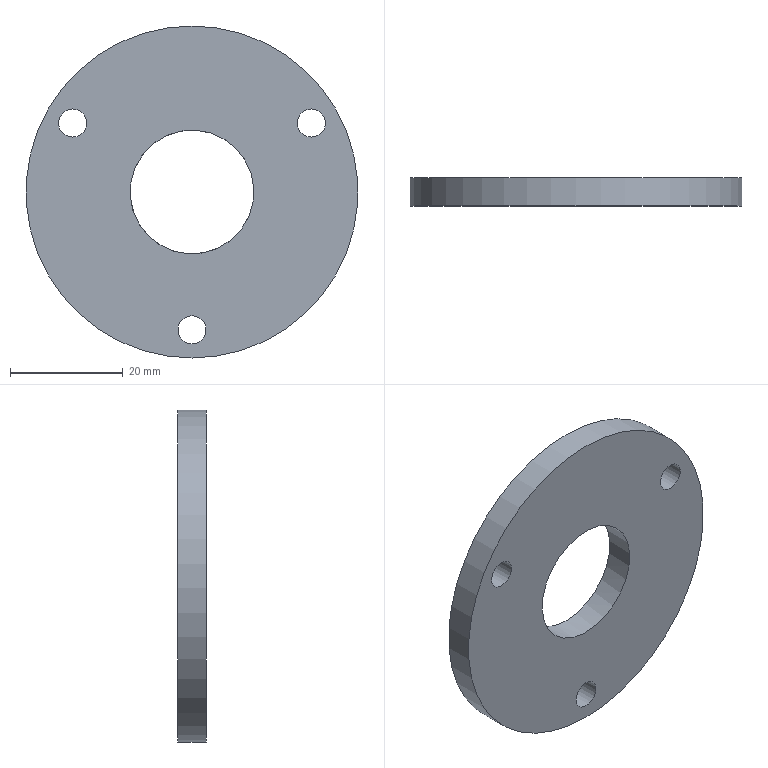Part | STEP file | YBQDJ-YB-14 | 1 solid | 7 faces | box 59 x 5 x 59 mm | volume 11475 mm3 | cylinder 5 | plane 2 | commonest cylinder face diameters 5 x3 22 x1 59 x1
STEP:
#1=CARTESIAN_POINT('',(0.,0.,0.));
#2=DIRECTION('',(0.,0.,1.));
#3=DIRECTION('',(1.,0.,0.));
#4=AXIS2_PLACEMENT_3D('',#1,#2,#3);
#5=CARTESIAN_POINT('',(51.5,-305.,130.5));
#6=VERTEX_POINT('',#5);
#7=CARTESIAN_POINT('',(51.5,-305.,101.));
#8=DIRECTION('',(0.,-1.,0.));
#9=DIRECTION('',(0.,0.,1.));
#10=AXIS2_PLACEMENT_3D('',#7,#8,#9);
#11=CIRCLE('',#10,29.5);
#12=CARTESIAN_POINT('',(51.5,-305.,101.));
#13=DIRECTION('',(0.,1.,0.));
#14=DIRECTION('',(-0.7071,0.,-0.7071));
#15=AXIS2_PLACEMENT_3D('',#12,#13,#14);
#16=CYLINDRICAL_SURFACE('',#15,29.5);
#17=CARTESIAN_POINT('',(8.639,0.));
#18=DIRECTION('',(-1.,0.));
#19=VECTOR('',#18,1.);
#20=LINE('',#17,#19);
#21=(GEOMETRIC_REPRESENTATION_CONTEXT(2)PARAMETRIC_REPRESENTATION_CONTEXT()REPRESENTATION_CONTEXT('',''));
#22=DEFINITIONAL_REPRESENTATION('',(#20),#21);
#23=PCURVE('',#16,#22);
#24=CARTESIAN_POINT('',(51.5,-305.,101.));
#25=DIRECTION('',(0.,1.,0.));
#26=DIRECTION('',(-0.7071,0.,-0.7071));
#27=AXIS2_PLACEMENT_3D('',#24,#25,#26);
#28=PLANE('',#27);
#29=CARTESIAN_POINT('',(-20.86,20.86));
#30=CARTESIAN_POINT('',(15.27,56.99));
#31=CARTESIAN_POINT('',(28.495,7.635));
#32=CARTESIAN_POINT('',(41.719,-41.719));
#33=CARTESIAN_POINT('',(-7.635,-28.495));
#34=CARTESIAN_POINT('',(-56.99,-15.27));
#35=CARTESIAN_POINT('',(-20.86,20.86));
#36=(BOUNDED_CURVE()B_SPLINE_CURVE(2,(#29,#30,#31,#32,#33,#34,#35),.UNSPECIFIED.,.T.,.F.)B_SPLINE_CURVE_WITH_KNOTS((1,2,2,2,2,1),(-2.094,0.,2.094,4.189,6.283,8.378),.UNSPECIFIED.)CURVE()GEOMETRIC_REPRESENTATION_ITEM()RATIONAL_B_SPLINE_CURVE((1.,0.5,1.,0.5,1.,0.5,1.))REPRESENTATION_ITEM(''));
#37=(GEOMETRIC_REPRESENTATION_CONTEXT(2)PARAMETRIC_REPRESENTATION_CONTEXT()REPRESENTATION_CONTEXT('',''));
#38=DEFINITIONAL_REPRESENTATION('',(#36),#37);
#39=PCURVE('',#28,#38);
#40=SURFACE_CURVE('',#11,(#23,#39),.PCURVE_S1.);
#41=EDGE_CURVE('',#6,#6,#40,.T.);
#42=ORIENTED_EDGE('',*,*,#41,.F.);
#43=CARTESIAN_POINT('',(51.5,-300.,130.5));
#44=VERTEX_POINT('',#43);
#45=CARTESIAN_POINT('',(51.5,-305.,130.5));
#46=CARTESIAN_POINT('',(51.5,-300.,130.5));
#47=B_SPLINE_CURVE_WITH_KNOTS('',1,(#45,#46),.UNSPECIFIED.,.F.,.F.,(2,2),(0.,5.),.PIECEWISE_BEZIER_KNOTS.);
#48=CARTESIAN_POINT('',(8.639,0.));
#49=DIRECTION('',(0.,1.));
#50=VECTOR('',#49,1.);
#51=LINE('',#48,#50);
#52=(GEOMETRIC_REPRESENTATION_CONTEXT(2)PARAMETRIC_REPRESENTATION_CONTEXT()REPRESENTATION_CONTEXT('',''));
#53=DEFINITIONAL_REPRESENTATION('',(#51),#52);
#54=PCURVE('',#16,#53);
#55=CARTESIAN_POINT('',(2.356,0.));
#56=DIRECTION('',(0.,1.));
#57=VECTOR('',#56,1.);
#58=LINE('',#55,#57);
#59=(GEOMETRIC_REPRESENTATION_CONTEXT(2)PARAMETRIC_REPRESENTATION_CONTEXT()REPRESENTATION_CONTEXT('',''));
#60=DEFINITIONAL_REPRESENTATION('',(#58),#59);
#61=PCURVE('',#16,#60);
#62=SEAM_CURVE('',#47,(#54,#61),.PCURVE_S1.);
#63=EDGE_CURVE('',#6,#44,#62,.T.);
#64=ORIENTED_EDGE('',*,*,#63,.T.);
#65=CARTESIAN_POINT('',(51.5,-300.,101.));
#66=DIRECTION('',(0.,-1.,0.));
#67=DIRECTION('',(0.,0.,1.));
#68=AXIS2_PLACEMENT_3D('',#65,#66,#67);
#69=CIRCLE('',#68,29.5);
#70=CARTESIAN_POINT('',(8.639,5.));
#71=DIRECTION('',(-1.,0.));
#72=VECTOR('',#71,1.);
#73=LINE('',#70,#72);
#74=(GEOMETRIC_REPRESENTATION_CONTEXT(2)PARAMETRIC_REPRESENTATION_CONTEXT()REPRESENTATION_CONTEXT('',''));
#75=DEFINITIONAL_REPRESENTATION('',(#73),#74);
#76=PCURVE('',#16,#75);
#77=CARTESIAN_POINT('',(-296.5,-300.,4.));
#78=DIRECTION('',(0.,-1.,0.));
#79=DIRECTION('',(0.,0.,-1.));
#80=AXIS2_PLACEMENT_3D('',#77,#78,#79);
#81=PLANE('',#80);
#82=CARTESIAN_POINT('',(-97.,348.));
#83=DIRECTION('',(-1.,0.));
#84=AXIS2_PLACEMENT_2D('',#82,#83);
#85=CIRCLE('',#84,29.5);
#86=(GEOMETRIC_REPRESENTATION_CONTEXT(2)PARAMETRIC_REPRESENTATION_CONTEXT()REPRESENTATION_CONTEXT('',''));
#87=DEFINITIONAL_REPRESENTATION('',(#85),#86);
#88=PCURVE('',#81,#87);
#89=SURFACE_CURVE('',#69,(#76,#88),.PCURVE_S1.);
#90=EDGE_CURVE('',#44,#44,#89,.T.);
#91=ORIENTED_EDGE('',*,*,#90,.T.);
#92=ORIENTED_EDGE('',*,*,#63,.F.);
#93=EDGE_LOOP('',(#42,#64,#91,#92));
#94=FACE_BOUND('',#93,.T.);
#95=ADVANCED_FACE('',(#94),#16,.T.);
#96=CARTESIAN_POINT('',(30.282,-305.,115.75));
#97=VERTEX_POINT('',#96);
#98=CARTESIAN_POINT('',(30.282,-305.,113.25));
#99=DIRECTION('',(0.,-1.,0.));
#100=DIRECTION('',(0.,0.,1.));
#101=AXIS2_PLACEMENT_3D('',#98,#99,#100);
#102=CIRCLE('',#101,2.5);
#103=CARTESIAN_POINT('',(4.573,25.433));
#104=CARTESIAN_POINT('',(7.635,28.495));
#105=CARTESIAN_POINT('',(8.756,24.312));
#106=CARTESIAN_POINT('',(9.877,20.13));
#107=CARTESIAN_POINT('',(5.694,21.25));
#108=CARTESIAN_POINT('',(1.511,22.371));
#109=CARTESIAN_POINT('',(4.573,25.433));
#110=(BOUNDED_CURVE()B_SPLINE_CURVE(2,(#103,#104,#105,#106,#107,#108,#109),.UNSPECIFIED.,.T.,.F.)B_SPLINE_CURVE_WITH_KNOTS((1,2,2,2,2,1),(-2.094,0.,2.094,4.189,6.283,8.378),.UNSPECIFIED.)CURVE()GEOMETRIC_REPRESENTATION_ITEM()RATIONAL_B_SPLINE_CURVE((1.,0.5,1.,0.5,1.,0.5,1.))REPRESENTATION_ITEM(''));
#111=(GEOMETRIC_REPRESENTATION_CONTEXT(2)PARAMETRIC_REPRESENTATION_CONTEXT()REPRESENTATION_CONTEXT('',''));
#112=DEFINITIONAL_REPRESENTATION('',(#110),#111);
#113=PCURVE('',#28,#112);
#114=CARTESIAN_POINT('',(30.282,-292.8,113.25));
#115=DIRECTION('',(0.,-1.,0.));
#116=DIRECTION('',(1.,0.,0.));
#117=AXIS2_PLACEMENT_3D('',#114,#115,#116);
#118=CYLINDRICAL_SURFACE('',#117,2.5);
#119=CARTESIAN_POINT('',(1.571,12.2));
#120=DIRECTION('',(1.,0.));
#121=VECTOR('',#120,1.);
#122=LINE('',#119,#121);
#123=(GEOMETRIC_REPRESENTATION_CONTEXT(2)PARAMETRIC_REPRESENTATION_CONTEXT()REPRESENTATION_CONTEXT('',''));
#124=DEFINITIONAL_REPRESENTATION('',(#122),#123);
#125=PCURVE('',#118,#124);
#126=SURFACE_CURVE('',#102,(#113,#125),.PCURVE_S1.);
#127=EDGE_CURVE('',#97,#97,#126,.T.);
#128=ORIENTED_EDGE('',*,*,#127,.F.);
#129=EDGE_LOOP('',(#128));
#130=FACE_BOUND('',#129,.T.);
#131=CARTESIAN_POINT('',(51.5,-305.,79.));
#132=VERTEX_POINT('',#131);
#133=CARTESIAN_POINT('',(51.5,-305.,76.5));
#134=DIRECTION('',(0.,-1.,0.));
#135=DIRECTION('',(0.,0.,1.));
#136=AXIS2_PLACEMENT_3D('',#133,#134,#135);
#137=CIRCLE('',#136,2.5);
#138=CARTESIAN_POINT('',(15.556,-15.556));
#139=CARTESIAN_POINT('',(18.618,-12.494));
#140=CARTESIAN_POINT('',(19.739,-16.677));
#141=CARTESIAN_POINT('',(20.86,-20.86));
#142=CARTESIAN_POINT('',(16.677,-19.739));
#143=CARTESIAN_POINT('',(12.494,-18.618));
#144=CARTESIAN_POINT('',(15.556,-15.556));
#145=(BOUNDED_CURVE()B_SPLINE_CURVE(2,(#138,#139,#140,#141,#142,#143,#144),.UNSPECIFIED.,.T.,.F.)B_SPLINE_CURVE_WITH_KNOTS((1,2,2,2,2,1),(-2.094,0.,2.094,4.189,6.283,8.378),.UNSPECIFIED.)CURVE()GEOMETRIC_REPRESENTATION_ITEM()RATIONAL_B_SPLINE_CURVE((1.,0.5,1.,0.5,1.,0.5,1.))REPRESENTATION_ITEM(''));
#146=(GEOMETRIC_REPRESENTATION_CONTEXT(2)PARAMETRIC_REPRESENTATION_CONTEXT()REPRESENTATION_CONTEXT('',''));
#147=DEFINITIONAL_REPRESENTATION('',(#145),#146);
#148=PCURVE('',#28,#147);
#149=CARTESIAN_POINT('',(51.5,-292.8,76.5));
#150=DIRECTION('',(0.,-1.,0.));
#151=DIRECTION('',(1.,0.,0.));
#152=AXIS2_PLACEMENT_3D('',#149,#150,#151);
#153=CYLINDRICAL_SURFACE('',#152,2.5);
#154=CARTESIAN_POINT('',(1.571,12.2));
#155=DIRECTION('',(1.,0.));
#156=VECTOR('',#155,1.);
#157=LINE('',#154,#156);
#158=(GEOMETRIC_REPRESENTATION_CONTEXT(2)PARAMETRIC_REPRESENTATION_CONTEXT()REPRESENTATION_CONTEXT('',''));
#159=DEFINITIONAL_REPRESENTATION('',(#157),#158);
#160=PCURVE('',#153,#159);
#161=SURFACE_CURVE('',#137,(#148,#160),.PCURVE_S1.);
#162=EDGE_CURVE('',#132,#132,#161,.T.);
#163=ORIENTED_EDGE('',*,*,#162,.F.);
#164=EDGE_LOOP('',(#163));
#165=FACE_BOUND('',#164,.T.);
#166=CARTESIAN_POINT('',(72.718,-305.,115.75));
#167=VERTEX_POINT('',#166);
#168=CARTESIAN_POINT('',(72.718,-305.,113.25));
#169=DIRECTION('',(0.,-1.,0.));
#170=DIRECTION('',(0.,0.,1.));
#171=AXIS2_PLACEMENT_3D('',#168,#169,#170);
#172=CIRCLE('',#171,2.5);
#173=CARTESIAN_POINT('',(-25.433,-4.573));
#174=CARTESIAN_POINT('',(-22.371,-1.511));
#175=CARTESIAN_POINT('',(-21.25,-5.694));
#176=CARTESIAN_POINT('',(-20.13,-9.877));
#177=CARTESIAN_POINT('',(-24.312,-8.756));
#178=CARTESIAN_POINT('',(-28.495,-7.635));
#179=CARTESIAN_POINT('',(-25.433,-4.573));
#180=(BOUNDED_CURVE()B_SPLINE_CURVE(2,(#173,#174,#175,#176,#177,#178,#179),.UNSPECIFIED.,.T.,.F.)B_SPLINE_CURVE_WITH_KNOTS((1,2,2,2,2,1),(-2.094,0.,2.094,4.189,6.283,8.378),.UNSPECIFIED.)CURVE()GEOMETRIC_REPRESENTATION_ITEM()RATIONAL_B_SPLINE_CURVE((1.,0.5,1.,0.5,1.,0.5,1.))REPRESENTATION_ITEM(''));
#181=(GEOMETRIC_REPRESENTATION_CONTEXT(2)PARAMETRIC_REPRESENTATION_CONTEXT()REPRESENTATION_CONTEXT('',''));
#182=DEFINITIONAL_REPRESENTATION('',(#180),#181);
#183=PCURVE('',#28,#182);
#184=CARTESIAN_POINT('',(72.718,-292.8,113.25));
#185=DIRECTION('',(0.,-1.,0.));
#186=DIRECTION('',(1.,0.,0.));
#187=AXIS2_PLACEMENT_3D('',#184,#185,#186);
#188=CYLINDRICAL_SURFACE('',#187,2.5);
#189=CARTESIAN_POINT('',(1.571,12.2));
#190=DIRECTION('',(1.,0.));
#191=VECTOR('',#190,1.);
#192=LINE('',#189,#191);
#193=(GEOMETRIC_REPRESENTATION_CONTEXT(2)PARAMETRIC_REPRESENTATION_CONTEXT()REPRESENTATION_CONTEXT('',''));
#194=DEFINITIONAL_REPRESENTATION('',(#192),#193);
#195=PCURVE('',#188,#194);
#196=SURFACE_CURVE('',#172,(#183,#195),.PCURVE_S1.);
#197=EDGE_CURVE('',#167,#167,#196,.T.);
#198=ORIENTED_EDGE('',*,*,#197,.F.);
#199=EDGE_LOOP('',(#198));
#200=FACE_BOUND('',#199,.T.);
#201=ORIENTED_EDGE('',*,*,#41,.T.);
#202=EDGE_LOOP('',(#201));
#203=FACE_BOUND('',#202,.T.);
#204=CARTESIAN_POINT('',(59.278,-305.,108.778));
#205=VERTEX_POINT('',#204);
#206=CARTESIAN_POINT('',(51.5,-305.,101.));
#207=DIRECTION('',(0.,1.,0.));
#208=DIRECTION('',(0.7071,0.,0.7071));
#209=AXIS2_PLACEMENT_3D('',#206,#207,#208);
#210=CIRCLE('',#209,11.);
#211=CARTESIAN_POINT('',(0.,0.));
#212=DIRECTION('',(-1.,0.));
#213=AXIS2_PLACEMENT_2D('',#211,#212);
#214=CIRCLE('',#213,11.);
#215=(GEOMETRIC_REPRESENTATION_CONTEXT(2)PARAMETRIC_REPRESENTATION_CONTEXT()REPRESENTATION_CONTEXT('',''));
#216=DEFINITIONAL_REPRESENTATION('',(#214),#215);
#217=PCURVE('',#28,#216);
#218=CARTESIAN_POINT('',(51.5,-295.,101.));
#219=DIRECTION('',(0.,-1.,0.));
#220=DIRECTION('',(0.7071,0.,0.7071));
#221=AXIS2_PLACEMENT_3D('',#218,#219,#220);
#222=CYLINDRICAL_SURFACE('',#221,11.);
#223=CARTESIAN_POINT('',(6.283,10.));
#224=DIRECTION('',(-1.,0.));
#225=VECTOR('',#224,1.);
#226=LINE('',#223,#225);
#227=(GEOMETRIC_REPRESENTATION_CONTEXT(2)PARAMETRIC_REPRESENTATION_CONTEXT()REPRESENTATION_CONTEXT('',''));
#228=DEFINITIONAL_REPRESENTATION('',(#226),#227);
#229=PCURVE('',#222,#228);
#230=SURFACE_CURVE('',#210,(#217,#229),.PCURVE_S1.);
#231=EDGE_CURVE('',#205,#205,#230,.T.);
#232=ORIENTED_EDGE('',*,*,#231,.T.);
#233=EDGE_LOOP('',(#232));
#234=FACE_BOUND('',#233,.T.);
#235=ADVANCED_FACE('',(#130,#165,#200,#203,#234),#28,.F.);
#236=CARTESIAN_POINT('',(51.5,-300.,90.));
#237=VERTEX_POINT('',#236);
#238=CARTESIAN_POINT('',(59.278,-300.,108.778));
#239=VERTEX_POINT('',#238);
#240=CARTESIAN_POINT('',(51.5,-300.,101.));
#241=DIRECTION('',(0.,1.,0.));
#242=DIRECTION('',(0.,0.,-1.));
#243=AXIS2_PLACEMENT_3D('',#240,#241,#242);
#244=CIRCLE('',#243,11.);
#245=CARTESIAN_POINT('',(-86.,348.));
#246=CARTESIAN_POINT('',(-86.,328.947));
#247=CARTESIAN_POINT('',(-102.5,338.474));
#248=CARTESIAN_POINT('',(-119.,348.));
#249=CARTESIAN_POINT('',(-102.5,357.526));
#250=CARTESIAN_POINT('',(-86.,367.053));
#251=CARTESIAN_POINT('',(-86.,348.));
#252=(BOUNDED_CURVE()B_SPLINE_CURVE(2,(#245,#246,#247,#248,#249,#250,#251),.UNSPECIFIED.,.T.,.F.)B_SPLINE_CURVE_WITH_KNOTS((1,2,2,2,2,1),(-2.094,0.,2.094,4.189,6.283,8.378),.UNSPECIFIED.)CURVE()GEOMETRIC_REPRESENTATION_ITEM()RATIONAL_B_SPLINE_CURVE((1.,0.5,1.,0.5,1.,0.5,1.))REPRESENTATION_ITEM(''));
#253=(GEOMETRIC_REPRESENTATION_CONTEXT(2)PARAMETRIC_REPRESENTATION_CONTEXT()REPRESENTATION_CONTEXT('',''));
#254=DEFINITIONAL_REPRESENTATION('',(#252),#253);
#255=PCURVE('',#81,#254);
#256=CARTESIAN_POINT('',(3.927,5.));
#257=DIRECTION('',(-1.,0.));
#258=VECTOR('',#257,1.);
#259=LINE('',#256,#258);
#260=(GEOMETRIC_REPRESENTATION_CONTEXT(2)PARAMETRIC_REPRESENTATION_CONTEXT()REPRESENTATION_CONTEXT('',''));
#261=DEFINITIONAL_REPRESENTATION('',(#259),#260);
#262=PCURVE('',#222,#261);
#263=SURFACE_CURVE('',#244,(#255,#262),.PCURVE_S1.);
#264=EDGE_CURVE('',#237,#239,#263,.T.);
#265=ORIENTED_EDGE('',*,*,#264,.F.);
#266=CARTESIAN_POINT('',(51.5,-300.,101.));
#267=DIRECTION('',(0.,1.,0.));
#268=DIRECTION('',(0.,0.,-1.));
#269=AXIS2_PLACEMENT_3D('',#266,#267,#268);
#270=CIRCLE('',#269,11.);
#271=CARTESIAN_POINT('',(-86.,348.));
#272=CARTESIAN_POINT('',(-86.,328.947));
#273=CARTESIAN_POINT('',(-102.5,338.474));
#274=CARTESIAN_POINT('',(-119.,348.));
#275=CARTESIAN_POINT('',(-102.5,357.526));
#276=CARTESIAN_POINT('',(-86.,367.053));
#277=CARTESIAN_POINT('',(-86.,348.));
#278=(BOUNDED_CURVE()B_SPLINE_CURVE(2,(#271,#272,#273,#274,#275,#276,#277),.UNSPECIFIED.,.T.,.F.)B_SPLINE_CURVE_WITH_KNOTS((1,2,2,2,2,1),(-2.094,0.,2.094,4.189,6.283,8.378),.UNSPECIFIED.)CURVE()GEOMETRIC_REPRESENTATION_ITEM()RATIONAL_B_SPLINE_CURVE((1.,0.5,1.,0.5,1.,0.5,1.))REPRESENTATION_ITEM(''));
#279=(GEOMETRIC_REPRESENTATION_CONTEXT(2)PARAMETRIC_REPRESENTATION_CONTEXT()REPRESENTATION_CONTEXT('',''));
#280=DEFINITIONAL_REPRESENTATION('',(#278),#279);
#281=PCURVE('',#81,#280);
#282=CARTESIAN_POINT('',(10.21,5.));
#283=DIRECTION('',(-1.,0.));
#284=VECTOR('',#283,1.);
#285=LINE('',#282,#284);
#286=(GEOMETRIC_REPRESENTATION_CONTEXT(2)PARAMETRIC_REPRESENTATION_CONTEXT()REPRESENTATION_CONTEXT('',''));
#287=DEFINITIONAL_REPRESENTATION('',(#285),#286);
#288=PCURVE('',#222,#287);
#289=SURFACE_CURVE('',#270,(#281,#288),.PCURVE_S1.);
#290=EDGE_CURVE('',#239,#237,#289,.T.);
#291=ORIENTED_EDGE('',*,*,#290,.F.);
#292=EDGE_LOOP('',(#265,#291));
#293=FACE_BOUND('',#292,.T.);
#294=CARTESIAN_POINT('',(30.282,-300.,115.75));
#295=VERTEX_POINT('',#294);
#296=CARTESIAN_POINT('',(30.282,-300.,113.25));
#297=DIRECTION('',(0.,-1.,0.));
#298=DIRECTION('',(0.,0.,1.));
#299=AXIS2_PLACEMENT_3D('',#296,#297,#298);
#300=CIRCLE('',#299,2.5);
#301=CARTESIAN_POINT('',(-109.25,326.782));
#302=DIRECTION('',(-1.,0.));
#303=AXIS2_PLACEMENT_2D('',#301,#302);
#304=CIRCLE('',#303,2.5);
#305=(GEOMETRIC_REPRESENTATION_CONTEXT(2)PARAMETRIC_REPRESENTATION_CONTEXT()REPRESENTATION_CONTEXT('',''));
#306=DEFINITIONAL_REPRESENTATION('',(#304),#305);
#307=PCURVE('',#81,#306);
#308=CARTESIAN_POINT('',(1.571,7.2));
#309=DIRECTION('',(1.,0.));
#310=VECTOR('',#309,1.);
#311=LINE('',#308,#310);
#312=(GEOMETRIC_REPRESENTATION_CONTEXT(2)PARAMETRIC_REPRESENTATION_CONTEXT()REPRESENTATION_CONTEXT('',''));
#313=DEFINITIONAL_REPRESENTATION('',(#311),#312);
#314=PCURVE('',#118,#313);
#315=SURFACE_CURVE('',#300,(#307,#314),.PCURVE_S1.);
#316=EDGE_CURVE('',#295,#295,#315,.T.);
#317=ORIENTED_EDGE('',*,*,#316,.T.);
#318=EDGE_LOOP('',(#317));
#319=FACE_BOUND('',#318,.T.);
#320=CARTESIAN_POINT('',(51.5,-300.,79.));
#321=VERTEX_POINT('',#320);
#322=CARTESIAN_POINT('',(51.5,-300.,76.5));
#323=DIRECTION('',(0.,-1.,0.));
#324=DIRECTION('',(0.,0.,1.));
#325=AXIS2_PLACEMENT_3D('',#322,#323,#324);
#326=CIRCLE('',#325,2.5);
#327=CARTESIAN_POINT('',(-72.5,348.));
#328=DIRECTION('',(-1.,0.));
#329=AXIS2_PLACEMENT_2D('',#327,#328);
#330=CIRCLE('',#329,2.5);
#331=(GEOMETRIC_REPRESENTATION_CONTEXT(2)PARAMETRIC_REPRESENTATION_CONTEXT()REPRESENTATION_CONTEXT('',''));
#332=DEFINITIONAL_REPRESENTATION('',(#330),#331);
#333=PCURVE('',#81,#332);
#334=CARTESIAN_POINT('',(1.571,7.2));
#335=DIRECTION('',(1.,0.));
#336=VECTOR('',#335,1.);
#337=LINE('',#334,#336);
#338=(GEOMETRIC_REPRESENTATION_CONTEXT(2)PARAMETRIC_REPRESENTATION_CONTEXT()REPRESENTATION_CONTEXT('',''));
#339=DEFINITIONAL_REPRESENTATION('',(#337),#338);
#340=PCURVE('',#153,#339);
#341=SURFACE_CURVE('',#326,(#333,#340),.PCURVE_S1.);
#342=EDGE_CURVE('',#321,#321,#341,.T.);
#343=ORIENTED_EDGE('',*,*,#342,.T.);
#344=EDGE_LOOP('',(#343));
#345=FACE_BOUND('',#344,.T.);
#346=CARTESIAN_POINT('',(72.718,-300.,115.75));
#347=VERTEX_POINT('',#346);
#348=CARTESIAN_POINT('',(72.718,-300.,113.25));
#349=DIRECTION('',(0.,-1.,0.));
#350=DIRECTION('',(0.,0.,1.));
#351=AXIS2_PLACEMENT_3D('',#348,#349,#350);
#352=CIRCLE('',#351,2.5);
#353=CARTESIAN_POINT('',(-109.25,369.218));
#354=DIRECTION('',(-1.,0.));
#355=AXIS2_PLACEMENT_2D('',#353,#354);
#356=CIRCLE('',#355,2.5);
#357=(GEOMETRIC_REPRESENTATION_CONTEXT(2)PARAMETRIC_REPRESENTATION_CONTEXT()REPRESENTATION_CONTEXT('',''));
#358=DEFINITIONAL_REPRESENTATION('',(#356),#357);
#359=PCURVE('',#81,#358);
#360=CARTESIAN_POINT('',(1.571,7.2));
#361=DIRECTION('',(1.,0.));
#362=VECTOR('',#361,1.);
#363=LINE('',#360,#362);
#364=(GEOMETRIC_REPRESENTATION_CONTEXT(2)PARAMETRIC_REPRESENTATION_CONTEXT()REPRESENTATION_CONTEXT('',''));
#365=DEFINITIONAL_REPRESENTATION('',(#363),#364);
#366=PCURVE('',#188,#365);
#367=SURFACE_CURVE('',#352,(#359,#366),.PCURVE_S1.);
#368=EDGE_CURVE('',#347,#347,#367,.T.);
#369=ORIENTED_EDGE('',*,*,#368,.T.);
#370=EDGE_LOOP('',(#369));
#371=FACE_BOUND('',#370,.T.);
#372=ORIENTED_EDGE('',*,*,#90,.F.);
#373=EDGE_LOOP('',(#372));
#374=FACE_BOUND('',#373,.T.);
#375=ADVANCED_FACE('',(#293,#319,#345,#371,#374),#81,.F.);
#376=ORIENTED_EDGE('',*,*,#290,.F.);
#377=CARTESIAN_POINT('',(59.278,-300.,108.778));
#378=CARTESIAN_POINT('',(59.278,-305.,108.778));
#379=B_SPLINE_CURVE_WITH_KNOTS('',1,(#377,#378),.UNSPECIFIED.,.F.,.F.,(2,2),(5.,10.),.PIECEWISE_BEZIER_KNOTS.);
#380=CARTESIAN_POINT('',(6.283,0.));
#381=DIRECTION('',(0.,1.));
#382=VECTOR('',#381,1.);
#383=LINE('',#380,#382);
#384=(GEOMETRIC_REPRESENTATION_CONTEXT(2)PARAMETRIC_REPRESENTATION_CONTEXT()REPRESENTATION_CONTEXT('',''));
#385=DEFINITIONAL_REPRESENTATION('',(#383),#384);
#386=PCURVE('',#222,#385);
#387=CARTESIAN_POINT('',(0.,0.));
#388=DIRECTION('',(0.,1.));
#389=VECTOR('',#388,1.);
#390=LINE('',#387,#389);
#391=(GEOMETRIC_REPRESENTATION_CONTEXT(2)PARAMETRIC_REPRESENTATION_CONTEXT()REPRESENTATION_CONTEXT('',''));
#392=DEFINITIONAL_REPRESENTATION('',(#390),#391);
#393=PCURVE('',#222,#392);
#394=SEAM_CURVE('',#379,(#386,#393),.PCURVE_S1.);
#395=EDGE_CURVE('',#239,#205,#394,.T.);
#396=ORIENTED_EDGE('',*,*,#395,.T.);
#397=ORIENTED_EDGE('',*,*,#231,.T.);
#398=ORIENTED_EDGE('',*,*,#395,.F.);
#399=ORIENTED_EDGE('',*,*,#264,.F.);
#400=EDGE_LOOP('',(#376,#396,#397,#398,#399));
#401=FACE_BOUND('',#400,.F.);
#402=ADVANCED_FACE('',(#401),#222,.F.);
#403=ORIENTED_EDGE('',*,*,#368,.T.);
#404=CARTESIAN_POINT('',(72.718,-300.,115.75));
#405=CARTESIAN_POINT('',(72.718,-305.,115.75));
#406=B_SPLINE_CURVE_WITH_KNOTS('',1,(#404,#405),.UNSPECIFIED.,.F.,.F.,(2,2),(7.2,12.2),.PIECEWISE_BEZIER_KNOTS.);
#407=CARTESIAN_POINT('',(7.854,0.));
#408=DIRECTION('',(0.,1.));
#409=VECTOR('',#408,1.);
#410=LINE('',#407,#409);
#411=(GEOMETRIC_REPRESENTATION_CONTEXT(2)PARAMETRIC_REPRESENTATION_CONTEXT()REPRESENTATION_CONTEXT('',''));
#412=DEFINITIONAL_REPRESENTATION('',(#410),#411);
#413=PCURVE('',#188,#412);
#414=CARTESIAN_POINT('',(1.571,0.));
#415=DIRECTION('',(0.,1.));
#416=VECTOR('',#415,1.);
#417=LINE('',#414,#416);
#418=(GEOMETRIC_REPRESENTATION_CONTEXT(2)PARAMETRIC_REPRESENTATION_CONTEXT()REPRESENTATION_CONTEXT('',''));
#419=DEFINITIONAL_REPRESENTATION('',(#417),#418);
#420=PCURVE('',#188,#419);
#421=SEAM_CURVE('',#406,(#413,#420),.PCURVE_S1.);
#422=EDGE_CURVE('',#347,#167,#421,.T.);
#423=ORIENTED_EDGE('',*,*,#422,.T.);
#424=ORIENTED_EDGE('',*,*,#197,.F.);
#425=ORIENTED_EDGE('',*,*,#422,.F.);
#426=EDGE_LOOP('',(#403,#423,#424,#425));
#427=FACE_BOUND('',#426,.F.);
#428=ADVANCED_FACE('',(#427),#188,.F.);
#429=ORIENTED_EDGE('',*,*,#342,.T.);
#430=CARTESIAN_POINT('',(51.5,-300.,79.));
#431=CARTESIAN_POINT('',(51.5,-305.,79.));
#432=B_SPLINE_CURVE_WITH_KNOTS('',1,(#430,#431),.UNSPECIFIED.,.F.,.F.,(2,2),(7.2,12.2),.PIECEWISE_BEZIER_KNOTS.);
#433=CARTESIAN_POINT('',(7.854,0.));
#434=DIRECTION('',(0.,1.));
#435=VECTOR('',#434,1.);
#436=LINE('',#433,#435);
#437=(GEOMETRIC_REPRESENTATION_CONTEXT(2)PARAMETRIC_REPRESENTATION_CONTEXT()REPRESENTATION_CONTEXT('',''));
#438=DEFINITIONAL_REPRESENTATION('',(#436),#437);
#439=PCURVE('',#153,#438);
#440=CARTESIAN_POINT('',(1.571,0.));
#441=DIRECTION('',(0.,1.));
#442=VECTOR('',#441,1.);
#443=LINE('',#440,#442);
#444=(GEOMETRIC_REPRESENTATION_CONTEXT(2)PARAMETRIC_REPRESENTATION_CONTEXT()REPRESENTATION_CONTEXT('',''));
#445=DEFINITIONAL_REPRESENTATION('',(#443),#444);
#446=PCURVE('',#153,#445);
#447=SEAM_CURVE('',#432,(#439,#446),.PCURVE_S1.);
#448=EDGE_CURVE('',#321,#132,#447,.T.);
#449=ORIENTED_EDGE('',*,*,#448,.T.);
#450=ORIENTED_EDGE('',*,*,#162,.F.);
#451=ORIENTED_EDGE('',*,*,#448,.F.);
#452=EDGE_LOOP('',(#429,#449,#450,#451));
#453=FACE_BOUND('',#452,.F.);
#454=ADVANCED_FACE('',(#453),#153,.F.);
#455=ORIENTED_EDGE('',*,*,#316,.T.);
#456=CARTESIAN_POINT('',(30.282,-300.,115.75));
#457=CARTESIAN_POINT('',(30.282,-305.,115.75));
#458=B_SPLINE_CURVE_WITH_KNOTS('',1,(#456,#457),.UNSPECIFIED.,.F.,.F.,(2,2),(7.2,12.2),.PIECEWISE_BEZIER_KNOTS.);
#459=CARTESIAN_POINT('',(7.854,0.));
#460=DIRECTION('',(0.,1.));
#461=VECTOR('',#460,1.);
#462=LINE('',#459,#461);
#463=(GEOMETRIC_REPRESENTATION_CONTEXT(2)PARAMETRIC_REPRESENTATION_CONTEXT()REPRESENTATION_CONTEXT('',''));
#464=DEFINITIONAL_REPRESENTATION('',(#462),#463);
#465=PCURVE('',#118,#464);
#466=CARTESIAN_POINT('',(1.571,0.));
#467=DIRECTION('',(0.,1.));
#468=VECTOR('',#467,1.);
#469=LINE('',#466,#468);
#470=(GEOMETRIC_REPRESENTATION_CONTEXT(2)PARAMETRIC_REPRESENTATION_CONTEXT()REPRESENTATION_CONTEXT('',''));
#471=DEFINITIONAL_REPRESENTATION('',(#469),#470);
#472=PCURVE('',#118,#471);
#473=SEAM_CURVE('',#458,(#465,#472),.PCURVE_S1.);
#474=EDGE_CURVE('',#295,#97,#473,.T.);
#475=ORIENTED_EDGE('',*,*,#474,.T.);
#476=ORIENTED_EDGE('',*,*,#127,.F.);
#477=ORIENTED_EDGE('',*,*,#474,.F.);
#478=EDGE_LOOP('',(#455,#475,#476,#477));
#479=FACE_BOUND('',#478,.F.);
#480=ADVANCED_FACE('',(#479),#118,.F.);
#481=CLOSED_SHELL('',(#95,#235,#375,#402,#428,#454,#480));
#482=MANIFOLD_SOLID_BREP('',#481);
#483=(LENGTH_UNIT()NAMED_UNIT(*)SI_UNIT(.MILLI.,.METRE.));
#484=UNCERTAINTY_MEASURE_WITH_UNIT(LENGTH_MEASURE(0.00001),#483,'','');
#485=(NAMED_UNIT(*)PLANE_ANGLE_UNIT()SI_UNIT($,.RADIAN.));
#486=(NAMED_UNIT(*)SI_UNIT($,.STERADIAN.)SOLID_ANGLE_UNIT());
#487=(GEOMETRIC_REPRESENTATION_CONTEXT(3)GLOBAL_UNCERTAINTY_ASSIGNED_CONTEXT((#484))GLOBAL_UNIT_ASSIGNED_CONTEXT((#483,#485,#486))REPRESENTATION_CONTEXT('',''));
#488=ADVANCED_BREP_SHAPE_REPRESENTATION('',(#4,#482),#487);